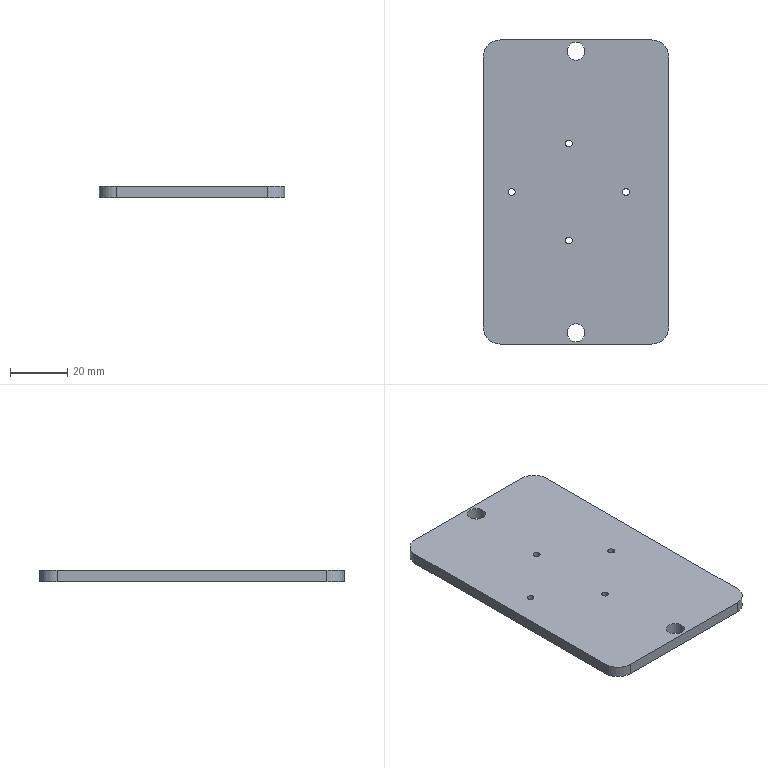Part | NX | features MOVE_FACE 2, DATUM_CSYS 1, EXTRUDE 1 | 1 solid | 16 faces | box 65 x 106.527 x 4 mm | volume 27252 mm3 | cylinder 10 | plane 6 | commonest cylinder face diameters 2.4 x4 12 x4 6.3 x2
STEP:
#1=CARTESIAN_POINT('',(4303.495,6820.373,0.));
#2=VERTEX_POINT('',#1);
#3=CARTESIAN_POINT('',(4303.495,6914.9,0.));
#4=VERTEX_POINT('',#3);
#5=CARTESIAN_POINT('',(4303.495,6818.473,0.));
#6=DIRECTION('',(0.,1.,0.));
#7=VECTOR('',#6,1000.);
#8=LINE('',#5,#7);
#9=EDGE_CURVE('',#2,#4,#8,.T.);
#10=ORIENTED_EDGE('',*,*,#9,.T.);
#11=CARTESIAN_POINT('',(4303.495,6914.9,-4.));
#12=VERTEX_POINT('',#11);
#13=CARTESIAN_POINT('',(4303.495,6914.9,-4.));
#14=DIRECTION('',(0.,0.,1.));
#15=VECTOR('',#14,1000.);
#16=LINE('',#13,#15);
#17=EDGE_CURVE('',#12,#4,#16,.T.);
#18=ORIENTED_EDGE('',*,*,#17,.F.);
#19=CARTESIAN_POINT('',(4303.495,6820.373,-4.));
#20=VERTEX_POINT('',#19);
#21=CARTESIAN_POINT('',(4303.495,6818.473,-4.));
#22=DIRECTION('',(0.,1.,0.));
#23=VECTOR('',#22,1000.);
#24=LINE('',#21,#23);
#25=EDGE_CURVE('',#20,#12,#24,.T.);
#26=ORIENTED_EDGE('',*,*,#25,.F.);
#27=CARTESIAN_POINT('',(4303.495,6820.373,-4.));
#28=DIRECTION('',(0.,0.,1.));
#29=VECTOR('',#28,1000.);
#30=LINE('',#27,#29);
#31=EDGE_CURVE('',#20,#2,#30,.T.);
#32=ORIENTED_EDGE('',*,*,#31,.T.);
#33=EDGE_LOOP('',(#10,#18,#26,#32));
#34=FACE_BOUND('',#33,.T.);
#35=CARTESIAN_POINT('',(4303.495,6818.473,-4.));
#36=DIRECTION('',(1.,0.,0.));
#37=DIRECTION('',(0.,0.,-1.));
#38=AXIS2_PLACEMENT_3D('',#35,#36,#37);
#39=PLANE('',#38);
#40=ADVANCED_FACE('',(#34),#39,.F.);
#41=CARTESIAN_POINT('',(4309.495,6920.9,0.));
#42=VERTEX_POINT('',#41);
#43=CARTESIAN_POINT('',(4309.495,6914.9,0.));
#44=DIRECTION('',(0.,0.,-1.));
#45=DIRECTION('',(1.,0.,0.));
#46=AXIS2_PLACEMENT_3D('',#43,#44,#45);
#47=CIRCLE('',#46,6.);
#48=EDGE_CURVE('',#4,#42,#47,.T.);
#49=ORIENTED_EDGE('',*,*,#48,.T.);
#50=CARTESIAN_POINT('',(4309.495,6920.9,-4.));
#51=VERTEX_POINT('',#50);
#52=CARTESIAN_POINT('',(4309.495,6920.9,-4.));
#53=DIRECTION('',(0.,0.,1.));
#54=VECTOR('',#53,1000.);
#55=LINE('',#52,#54);
#56=EDGE_CURVE('',#51,#42,#55,.T.);
#57=ORIENTED_EDGE('',*,*,#56,.F.);
#58=CARTESIAN_POINT('',(4309.495,6914.9,-4.));
#59=DIRECTION('',(0.,0.,-1.));
#60=DIRECTION('',(1.,0.,0.));
#61=AXIS2_PLACEMENT_3D('',#58,#59,#60);
#62=CIRCLE('',#61,6.);
#63=EDGE_CURVE('',#12,#51,#62,.T.);
#64=ORIENTED_EDGE('',*,*,#63,.F.);
#65=ORIENTED_EDGE('',*,*,#17,.T.);
#66=EDGE_LOOP('',(#49,#57,#64,#65));
#67=FACE_BOUND('',#66,.T.);
#68=CARTESIAN_POINT('',(4309.495,6914.9,-4.));
#69=DIRECTION('',(0.,0.,1.));
#70=DIRECTION('',(1.,0.,0.));
#71=AXIS2_PLACEMENT_3D('',#68,#69,#70);
#72=CYLINDRICAL_SURFACE('',#71,6.);
#73=ADVANCED_FACE('',(#67),#72,.T.);
#74=CARTESIAN_POINT('',(4362.495,6920.9,0.));
#75=VERTEX_POINT('',#74);
#76=CARTESIAN_POINT('',(4309.495,6920.9,0.));
#77=DIRECTION('',(1.,0.,0.));
#78=VECTOR('',#77,1000.);
#79=LINE('',#76,#78);
#80=EDGE_CURVE('',#42,#75,#79,.T.);
#81=ORIENTED_EDGE('',*,*,#80,.T.);
#82=CARTESIAN_POINT('',(4362.495,6920.9,-4.));
#83=VERTEX_POINT('',#82);
#84=CARTESIAN_POINT('',(4362.495,6920.9,-4.));
#85=DIRECTION('',(0.,0.,1.));
#86=VECTOR('',#85,1000.);
#87=LINE('',#84,#86);
#88=EDGE_CURVE('',#83,#75,#87,.T.);
#89=ORIENTED_EDGE('',*,*,#88,.F.);
#90=CARTESIAN_POINT('',(4309.495,6920.9,-4.));
#91=DIRECTION('',(1.,0.,0.));
#92=VECTOR('',#91,1000.);
#93=LINE('',#90,#92);
#94=EDGE_CURVE('',#51,#83,#93,.T.);
#95=ORIENTED_EDGE('',*,*,#94,.F.);
#96=ORIENTED_EDGE('',*,*,#56,.T.);
#97=EDGE_LOOP('',(#81,#89,#95,#96));
#98=FACE_BOUND('',#97,.T.);
#99=CARTESIAN_POINT('',(4309.495,6920.9,-4.));
#100=DIRECTION('',(0.,-1.,0.));
#101=DIRECTION('',(0.,0.,-1.));
#102=AXIS2_PLACEMENT_3D('',#99,#100,#101);
#103=PLANE('',#102);
#104=ADVANCED_FACE('',(#98),#103,.F.);
#105=CARTESIAN_POINT('',(4368.495,6914.9,0.));
#106=VERTEX_POINT('',#105);
#107=CARTESIAN_POINT('',(4362.495,6914.9,0.));
#108=DIRECTION('',(0.,0.,-1.));
#109=DIRECTION('',(1.,0.,0.));
#110=AXIS2_PLACEMENT_3D('',#107,#108,#109);
#111=CIRCLE('',#110,6.);
#112=EDGE_CURVE('',#75,#106,#111,.T.);
#113=ORIENTED_EDGE('',*,*,#112,.T.);
#114=CARTESIAN_POINT('',(4368.495,6914.9,-4.));
#115=VERTEX_POINT('',#114);
#116=CARTESIAN_POINT('',(4368.495,6914.9,-4.));
#117=DIRECTION('',(0.,0.,1.));
#118=VECTOR('',#117,1000.);
#119=LINE('',#116,#118);
#120=EDGE_CURVE('',#115,#106,#119,.T.);
#121=ORIENTED_EDGE('',*,*,#120,.F.);
#122=CARTESIAN_POINT('',(4362.495,6914.9,-4.));
#123=DIRECTION('',(0.,0.,-1.));
#124=DIRECTION('',(1.,0.,0.));
#125=AXIS2_PLACEMENT_3D('',#122,#123,#124);
#126=CIRCLE('',#125,6.);
#127=EDGE_CURVE('',#83,#115,#126,.T.);
#128=ORIENTED_EDGE('',*,*,#127,.F.);
#129=ORIENTED_EDGE('',*,*,#88,.T.);
#130=EDGE_LOOP('',(#113,#121,#128,#129));
#131=FACE_BOUND('',#130,.T.);
#132=CARTESIAN_POINT('',(4362.495,6914.9,-4.));
#133=DIRECTION('',(0.,0.,1.));
#134=DIRECTION('',(1.,0.,0.));
#135=AXIS2_PLACEMENT_3D('',#132,#133,#134);
#136=CYLINDRICAL_SURFACE('',#135,6.);
#137=ADVANCED_FACE('',(#131),#136,.T.);
#138=CARTESIAN_POINT('',(4368.495,6820.373,0.));
#139=VERTEX_POINT('',#138);
#140=CARTESIAN_POINT('',(4368.495,6916.8,0.));
#141=DIRECTION('',(0.,-1.,0.));
#142=VECTOR('',#141,1000.);
#143=LINE('',#140,#142);
#144=EDGE_CURVE('',#106,#139,#143,.T.);
#145=ORIENTED_EDGE('',*,*,#144,.T.);
#146=CARTESIAN_POINT('',(4368.495,6820.373,-4.));
#147=VERTEX_POINT('',#146);
#148=CARTESIAN_POINT('',(4368.495,6820.373,-4.));
#149=DIRECTION('',(0.,0.,1.));
#150=VECTOR('',#149,1000.);
#151=LINE('',#148,#150);
#152=EDGE_CURVE('',#147,#139,#151,.T.);
#153=ORIENTED_EDGE('',*,*,#152,.F.);
#154=CARTESIAN_POINT('',(4368.495,6916.8,-4.));
#155=DIRECTION('',(0.,-1.,0.));
#156=VECTOR('',#155,1000.);
#157=LINE('',#154,#156);
#158=EDGE_CURVE('',#115,#147,#157,.T.);
#159=ORIENTED_EDGE('',*,*,#158,.F.);
#160=ORIENTED_EDGE('',*,*,#120,.T.);
#161=EDGE_LOOP('',(#145,#153,#159,#160));
#162=FACE_BOUND('',#161,.T.);
#163=CARTESIAN_POINT('',(4368.495,6916.8,-4.));
#164=DIRECTION('',(-1.,0.,0.));
#165=DIRECTION('',(0.,0.,1.));
#166=AXIS2_PLACEMENT_3D('',#163,#164,#165);
#167=PLANE('',#166);
#168=ADVANCED_FACE('',(#162),#167,.F.);
#169=CARTESIAN_POINT('',(4362.495,6814.373,0.));
#170=VERTEX_POINT('',#169);
#171=CARTESIAN_POINT('',(4362.495,6820.373,0.));
#172=DIRECTION('',(0.,0.,-1.));
#173=DIRECTION('',(1.,0.,0.));
#174=AXIS2_PLACEMENT_3D('',#171,#172,#173);
#175=CIRCLE('',#174,6.);
#176=EDGE_CURVE('',#139,#170,#175,.T.);
#177=ORIENTED_EDGE('',*,*,#176,.T.);
#178=CARTESIAN_POINT('',(4362.495,6814.373,-4.));
#179=VERTEX_POINT('',#178);
#180=CARTESIAN_POINT('',(4362.495,6814.373,-4.));
#181=DIRECTION('',(0.,0.,1.));
#182=VECTOR('',#181,1000.);
#183=LINE('',#180,#182);
#184=EDGE_CURVE('',#179,#170,#183,.T.);
#185=ORIENTED_EDGE('',*,*,#184,.F.);
#186=CARTESIAN_POINT('',(4362.495,6820.373,-4.));
#187=DIRECTION('',(0.,0.,-1.));
#188=DIRECTION('',(1.,0.,0.));
#189=AXIS2_PLACEMENT_3D('',#186,#187,#188);
#190=CIRCLE('',#189,6.);
#191=EDGE_CURVE('',#147,#179,#190,.T.);
#192=ORIENTED_EDGE('',*,*,#191,.F.);
#193=ORIENTED_EDGE('',*,*,#152,.T.);
#194=EDGE_LOOP('',(#177,#185,#192,#193));
#195=FACE_BOUND('',#194,.T.);
#196=CARTESIAN_POINT('',(4362.495,6820.373,-4.));
#197=DIRECTION('',(0.,0.,1.));
#198=DIRECTION('',(1.,0.,0.));
#199=AXIS2_PLACEMENT_3D('',#196,#197,#198);
#200=CYLINDRICAL_SURFACE('',#199,6.);
#201=ADVANCED_FACE('',(#195),#200,.T.);
#202=CARTESIAN_POINT('',(4309.495,6814.373,0.));
#203=VERTEX_POINT('',#202);
#204=CARTESIAN_POINT('',(4362.495,6814.373,0.));
#205=DIRECTION('',(-1.,0.,0.));
#206=VECTOR('',#205,1000.);
#207=LINE('',#204,#206);
#208=EDGE_CURVE('',#170,#203,#207,.T.);
#209=ORIENTED_EDGE('',*,*,#208,.T.);
#210=CARTESIAN_POINT('',(4309.495,6814.373,-4.));
#211=VERTEX_POINT('',#210);
#212=CARTESIAN_POINT('',(4309.495,6814.373,-4.));
#213=DIRECTION('',(0.,0.,1.));
#214=VECTOR('',#213,1000.);
#215=LINE('',#212,#214);
#216=EDGE_CURVE('',#211,#203,#215,.T.);
#217=ORIENTED_EDGE('',*,*,#216,.F.);
#218=CARTESIAN_POINT('',(4362.495,6814.373,-4.));
#219=DIRECTION('',(-1.,0.,0.));
#220=VECTOR('',#219,1000.);
#221=LINE('',#218,#220);
#222=EDGE_CURVE('',#179,#211,#221,.T.);
#223=ORIENTED_EDGE('',*,*,#222,.F.);
#224=ORIENTED_EDGE('',*,*,#184,.T.);
#225=EDGE_LOOP('',(#209,#217,#223,#224));
#226=FACE_BOUND('',#225,.T.);
#227=CARTESIAN_POINT('',(4362.495,6814.373,-4.));
#228=DIRECTION('',(0.,1.,0.));
#229=DIRECTION('',(0.,0.,1.));
#230=AXIS2_PLACEMENT_3D('',#227,#228,#229);
#231=PLANE('',#230);
#232=ADVANCED_FACE('',(#226),#231,.F.);
#233=CARTESIAN_POINT('',(4334.695,6850.637,-4.));
#234=VERTEX_POINT('',#233);
#235=CARTESIAN_POINT('',(4333.495,6850.637,-4.));
#236=DIRECTION('',(0.,0.,1.));
#237=DIRECTION('',(1.,0.,0.));
#238=AXIS2_PLACEMENT_3D('',#235,#236,#237);
#239=CIRCLE('',#238,1.2);
#240=EDGE_CURVE('',#234,#234,#239,.T.);
#241=ORIENTED_EDGE('',*,*,#240,.F.);
#242=EDGE_LOOP('',(#241));
#243=FACE_BOUND('',#242,.T.);
#244=CARTESIAN_POINT('',(4334.695,6850.637,0.));
#245=VERTEX_POINT('',#244);
#246=CARTESIAN_POINT('',(4333.495,6850.637,0.));
#247=DIRECTION('',(0.,0.,1.));
#248=DIRECTION('',(1.,0.,0.));
#249=AXIS2_PLACEMENT_3D('',#246,#247,#248);
#250=CIRCLE('',#249,1.2);
#251=EDGE_CURVE('',#245,#245,#250,.T.);
#252=ORIENTED_EDGE('',*,*,#251,.T.);
#253=EDGE_LOOP('',(#252));
#254=FACE_BOUND('',#253,.T.);
#255=CARTESIAN_POINT('',(4333.495,6850.637,-4.));
#256=DIRECTION('',(0.,0.,1.));
#257=DIRECTION('',(1.,0.,0.));
#258=AXIS2_PLACEMENT_3D('',#255,#256,#257);
#259=CYLINDRICAL_SURFACE('',#258,1.2);
#260=ADVANCED_FACE('',(#243,#254),#259,.F.);
#261=CARTESIAN_POINT('',(4334.695,6884.637,-4.));
#262=VERTEX_POINT('',#261);
#263=CARTESIAN_POINT('',(4333.495,6884.637,-4.));
#264=DIRECTION('',(0.,0.,1.));
#265=DIRECTION('',(1.,0.,0.));
#266=AXIS2_PLACEMENT_3D('',#263,#264,#265);
#267=CIRCLE('',#266,1.2);
#268=EDGE_CURVE('',#262,#262,#267,.T.);
#269=ORIENTED_EDGE('',*,*,#268,.F.);
#270=EDGE_LOOP('',(#269));
#271=FACE_BOUND('',#270,.T.);
#272=CARTESIAN_POINT('',(4334.695,6884.637,0.));
#273=VERTEX_POINT('',#272);
#274=CARTESIAN_POINT('',(4333.495,6884.637,0.));
#275=DIRECTION('',(0.,0.,1.));
#276=DIRECTION('',(1.,0.,0.));
#277=AXIS2_PLACEMENT_3D('',#274,#275,#276);
#278=CIRCLE('',#277,1.2);
#279=EDGE_CURVE('',#273,#273,#278,.T.);
#280=ORIENTED_EDGE('',*,*,#279,.T.);
#281=EDGE_LOOP('',(#280));
#282=FACE_BOUND('',#281,.T.);
#283=CARTESIAN_POINT('',(4333.495,6884.637,-4.));
#284=DIRECTION('',(0.,0.,1.));
#285=DIRECTION('',(1.,0.,0.));
#286=AXIS2_PLACEMENT_3D('',#283,#284,#285);
#287=CYLINDRICAL_SURFACE('',#286,1.2);
#288=ADVANCED_FACE('',(#271,#282),#287,.F.);
#289=CARTESIAN_POINT('',(4339.145,6818.368,-4.));
#290=VERTEX_POINT('',#289);
#291=CARTESIAN_POINT('',(4335.995,6818.368,-4.));
#292=DIRECTION('',(0.,0.,1.));
#293=DIRECTION('',(1.,0.,0.));
#294=AXIS2_PLACEMENT_3D('',#291,#292,#293);
#295=CIRCLE('',#294,3.15);
#296=EDGE_CURVE('',#290,#290,#295,.T.);
#297=ORIENTED_EDGE('',*,*,#296,.F.);
#298=EDGE_LOOP('',(#297));
#299=FACE_BOUND('',#298,.T.);
#300=CARTESIAN_POINT('',(4339.145,6818.368,0.));
#301=VERTEX_POINT('',#300);
#302=CARTESIAN_POINT('',(4335.995,6818.368,0.));
#303=DIRECTION('',(0.,0.,1.));
#304=DIRECTION('',(1.,0.,0.));
#305=AXIS2_PLACEMENT_3D('',#302,#303,#304);
#306=CIRCLE('',#305,3.15);
#307=EDGE_CURVE('',#301,#301,#306,.T.);
#308=ORIENTED_EDGE('',*,*,#307,.T.);
#309=EDGE_LOOP('',(#308));
#310=FACE_BOUND('',#309,.T.);
#311=CARTESIAN_POINT('',(4335.995,6818.368,-4.));
#312=DIRECTION('',(0.,0.,1.));
#313=DIRECTION('',(1.,0.,0.));
#314=AXIS2_PLACEMENT_3D('',#311,#312,#313);
#315=CYLINDRICAL_SURFACE('',#314,3.15);
#316=ADVANCED_FACE('',(#299,#310),#315,.F.);
#317=CARTESIAN_POINT('',(4339.145,6916.905,-4.));
#318=VERTEX_POINT('',#317);
#319=CARTESIAN_POINT('',(4335.995,6916.905,-4.));
#320=DIRECTION('',(0.,0.,1.));
#321=DIRECTION('',(1.,0.,0.));
#322=AXIS2_PLACEMENT_3D('',#319,#320,#321);
#323=CIRCLE('',#322,3.15);
#324=EDGE_CURVE('',#318,#318,#323,.T.);
#325=ORIENTED_EDGE('',*,*,#324,.F.);
#326=EDGE_LOOP('',(#325));
#327=FACE_BOUND('',#326,.T.);
#328=CARTESIAN_POINT('',(4339.145,6916.905,0.));
#329=VERTEX_POINT('',#328);
#330=CARTESIAN_POINT('',(4335.995,6916.905,0.));
#331=DIRECTION('',(0.,0.,1.));
#332=DIRECTION('',(1.,0.,0.));
#333=AXIS2_PLACEMENT_3D('',#330,#331,#332);
#334=CIRCLE('',#333,3.15);
#335=EDGE_CURVE('',#329,#329,#334,.T.);
#336=ORIENTED_EDGE('',*,*,#335,.T.);
#337=EDGE_LOOP('',(#336));
#338=FACE_BOUND('',#337,.T.);
#339=CARTESIAN_POINT('',(4335.995,6916.905,-4.));
#340=DIRECTION('',(0.,0.,1.));
#341=DIRECTION('',(1.,0.,0.));
#342=AXIS2_PLACEMENT_3D('',#339,#340,#341);
#343=CYLINDRICAL_SURFACE('',#342,3.15);
#344=ADVANCED_FACE('',(#327,#338),#343,.F.);
#345=CARTESIAN_POINT('',(4354.695,6867.637,-4.));
#346=VERTEX_POINT('',#345);
#347=CARTESIAN_POINT('',(4353.495,6867.637,-4.));
#348=DIRECTION('',(0.,0.,1.));
#349=DIRECTION('',(1.,0.,0.));
#350=AXIS2_PLACEMENT_3D('',#347,#348,#349);
#351=CIRCLE('',#350,1.2);
#352=EDGE_CURVE('',#346,#346,#351,.T.);
#353=ORIENTED_EDGE('',*,*,#352,.F.);
#354=EDGE_LOOP('',(#353));
#355=FACE_BOUND('',#354,.T.);
#356=CARTESIAN_POINT('',(4354.695,6867.637,0.));
#357=VERTEX_POINT('',#356);
#358=CARTESIAN_POINT('',(4353.495,6867.637,0.));
#359=DIRECTION('',(0.,0.,1.));
#360=DIRECTION('',(1.,0.,0.));
#361=AXIS2_PLACEMENT_3D('',#358,#359,#360);
#362=CIRCLE('',#361,1.2);
#363=EDGE_CURVE('',#357,#357,#362,.T.);
#364=ORIENTED_EDGE('',*,*,#363,.T.);
#365=EDGE_LOOP('',(#364));
#366=FACE_BOUND('',#365,.T.);
#367=CARTESIAN_POINT('',(4353.495,6867.637,-4.));
#368=DIRECTION('',(0.,0.,1.));
#369=DIRECTION('',(1.,0.,0.));
#370=AXIS2_PLACEMENT_3D('',#367,#368,#369);
#371=CYLINDRICAL_SURFACE('',#370,1.2);
#372=ADVANCED_FACE('',(#355,#366),#371,.F.);
#373=CARTESIAN_POINT('',(4309.495,6820.373,0.));
#374=DIRECTION('',(0.,0.,-1.));
#375=DIRECTION('',(1.,0.,0.));
#376=AXIS2_PLACEMENT_3D('',#373,#374,#375);
#377=CIRCLE('',#376,6.);
#378=EDGE_CURVE('',#203,#2,#377,.T.);
#379=ORIENTED_EDGE('',*,*,#378,.T.);
#380=ORIENTED_EDGE('',*,*,#31,.F.);
#381=CARTESIAN_POINT('',(4309.495,6820.373,-4.));
#382=DIRECTION('',(0.,0.,-1.));
#383=DIRECTION('',(1.,0.,0.));
#384=AXIS2_PLACEMENT_3D('',#381,#382,#383);
#385=CIRCLE('',#384,6.);
#386=EDGE_CURVE('',#211,#20,#385,.T.);
#387=ORIENTED_EDGE('',*,*,#386,.F.);
#388=ORIENTED_EDGE('',*,*,#216,.T.);
#389=EDGE_LOOP('',(#379,#380,#387,#388));
#390=FACE_BOUND('',#389,.T.);
#391=CARTESIAN_POINT('',(4309.495,6820.373,-4.));
#392=DIRECTION('',(0.,0.,1.));
#393=DIRECTION('',(1.,0.,0.));
#394=AXIS2_PLACEMENT_3D('',#391,#392,#393);
#395=CYLINDRICAL_SURFACE('',#394,6.);
#396=ADVANCED_FACE('',(#390),#395,.T.);
#397=CARTESIAN_POINT('',(4314.695,6867.637,-4.));
#398=VERTEX_POINT('',#397);
#399=CARTESIAN_POINT('',(4313.495,6867.637,-4.));
#400=DIRECTION('',(0.,0.,1.));
#401=DIRECTION('',(1.,0.,0.));
#402=AXIS2_PLACEMENT_3D('',#399,#400,#401);
#403=CIRCLE('',#402,1.2);
#404=EDGE_CURVE('',#398,#398,#403,.T.);
#405=ORIENTED_EDGE('',*,*,#404,.F.);
#406=EDGE_LOOP('',(#405));
#407=FACE_BOUND('',#406,.T.);
#408=CARTESIAN_POINT('',(4314.695,6867.637,0.));
#409=VERTEX_POINT('',#408);
#410=CARTESIAN_POINT('',(4313.495,6867.637,0.));
#411=DIRECTION('',(0.,0.,1.));
#412=DIRECTION('',(1.,0.,0.));
#413=AXIS2_PLACEMENT_3D('',#410,#411,#412);
#414=CIRCLE('',#413,1.2);
#415=EDGE_CURVE('',#409,#409,#414,.T.);
#416=ORIENTED_EDGE('',*,*,#415,.T.);
#417=EDGE_LOOP('',(#416));
#418=FACE_BOUND('',#417,.T.);
#419=CARTESIAN_POINT('',(4313.495,6867.637,-4.));
#420=DIRECTION('',(0.,0.,1.));
#421=DIRECTION('',(1.,0.,0.));
#422=AXIS2_PLACEMENT_3D('',#419,#420,#421);
#423=CYLINDRICAL_SURFACE('',#422,1.2);
#424=ADVANCED_FACE('',(#407,#418),#423,.F.);
#425=ORIENTED_EDGE('',*,*,#25,.T.);
#426=ORIENTED_EDGE('',*,*,#63,.T.);
#427=ORIENTED_EDGE('',*,*,#94,.T.);
#428=ORIENTED_EDGE('',*,*,#127,.T.);
#429=ORIENTED_EDGE('',*,*,#158,.T.);
#430=ORIENTED_EDGE('',*,*,#191,.T.);
#431=ORIENTED_EDGE('',*,*,#222,.T.);
#432=ORIENTED_EDGE('',*,*,#386,.T.);
#433=EDGE_LOOP('',(#425,#426,#427,#428,#429,#430,#431,#432));
#434=FACE_BOUND('',#433,.T.);
#435=ORIENTED_EDGE('',*,*,#352,.T.);
#436=EDGE_LOOP('',(#435));
#437=FACE_BOUND('',#436,.T.);
#438=ORIENTED_EDGE('',*,*,#324,.T.);
#439=EDGE_LOOP('',(#438));
#440=FACE_BOUND('',#439,.T.);
#441=ORIENTED_EDGE('',*,*,#296,.T.);
#442=EDGE_LOOP('',(#441));
#443=FACE_BOUND('',#442,.T.);
#444=ORIENTED_EDGE('',*,*,#268,.T.);
#445=EDGE_LOOP('',(#444));
#446=FACE_BOUND('',#445,.T.);
#447=ORIENTED_EDGE('',*,*,#240,.T.);
#448=EDGE_LOOP('',(#447));
#449=FACE_BOUND('',#448,.T.);
#450=ORIENTED_EDGE('',*,*,#404,.T.);
#451=EDGE_LOOP('',(#450));
#452=FACE_BOUND('',#451,.T.);
#453=CARTESIAN_POINT('',(4309.495,6916.8,-4.));
#454=DIRECTION('',(0.,0.,-1.));
#455=DIRECTION('',(-1.,0.,0.));
#456=AXIS2_PLACEMENT_3D('',#453,#454,#455);
#457=PLANE('',#456);
#458=ADVANCED_FACE('',(#434,#437,#440,#443,#446,#449,#452),#457,.T.);
#459=ORIENTED_EDGE('',*,*,#9,.F.);
#460=ORIENTED_EDGE('',*,*,#378,.F.);
#461=ORIENTED_EDGE('',*,*,#208,.F.);
#462=ORIENTED_EDGE('',*,*,#176,.F.);
#463=ORIENTED_EDGE('',*,*,#144,.F.);
#464=ORIENTED_EDGE('',*,*,#112,.F.);
#465=ORIENTED_EDGE('',*,*,#80,.F.);
#466=ORIENTED_EDGE('',*,*,#48,.F.);
#467=EDGE_LOOP('',(#459,#460,#461,#462,#463,#464,#465,#466));
#468=FACE_BOUND('',#467,.T.);
#469=ORIENTED_EDGE('',*,*,#363,.F.);
#470=EDGE_LOOP('',(#469));
#471=FACE_BOUND('',#470,.T.);
#472=ORIENTED_EDGE('',*,*,#335,.F.);
#473=EDGE_LOOP('',(#472));
#474=FACE_BOUND('',#473,.T.);
#475=ORIENTED_EDGE('',*,*,#307,.F.);
#476=EDGE_LOOP('',(#475));
#477=FACE_BOUND('',#476,.T.);
#478=ORIENTED_EDGE('',*,*,#279,.F.);
#479=EDGE_LOOP('',(#478));
#480=FACE_BOUND('',#479,.T.);
#481=ORIENTED_EDGE('',*,*,#251,.F.);
#482=EDGE_LOOP('',(#481));
#483=FACE_BOUND('',#482,.T.);
#484=ORIENTED_EDGE('',*,*,#415,.F.);
#485=EDGE_LOOP('',(#484));
#486=FACE_BOUND('',#485,.T.);
#487=CARTESIAN_POINT('',(4309.495,6916.8,0.));
#488=DIRECTION('',(0.,0.,-1.));
#489=DIRECTION('',(-1.,0.,0.));
#490=AXIS2_PLACEMENT_3D('',#487,#488,#489);
#491=PLANE('',#490);
#492=ADVANCED_FACE('',(#468,#471,#474,#477,#480,#483,#486),#491,.F.);
#493=CLOSED_SHELL('',(#40,#73,#104,#137,#168,#201,#232,#260,#288,#316,#344,#372,#396,#424,#458,#492));
#494=MANIFOLD_SOLID_BREP('',#493);
#495=(LENGTH_UNIT()NAMED_UNIT(*)SI_UNIT(.MILLI.,.METRE.));
#496=UNCERTAINTY_MEASURE_WITH_UNIT(LENGTH_MEASURE(0.00001),#495,'','');
#497=(NAMED_UNIT(*)PLANE_ANGLE_UNIT()SI_UNIT($,.RADIAN.));
#498=(NAMED_UNIT(*)SI_UNIT($,.STERADIAN.)SOLID_ANGLE_UNIT());
#499=(GEOMETRIC_REPRESENTATION_CONTEXT(3)GLOBAL_UNCERTAINTY_ASSIGNED_CONTEXT((#496))GLOBAL_UNIT_ASSIGNED_CONTEXT((#495,#497,#498))REPRESENTATION_CONTEXT('',''));
#500=ADVANCED_BREP_SHAPE_REPRESENTATION('',(#494),#499);